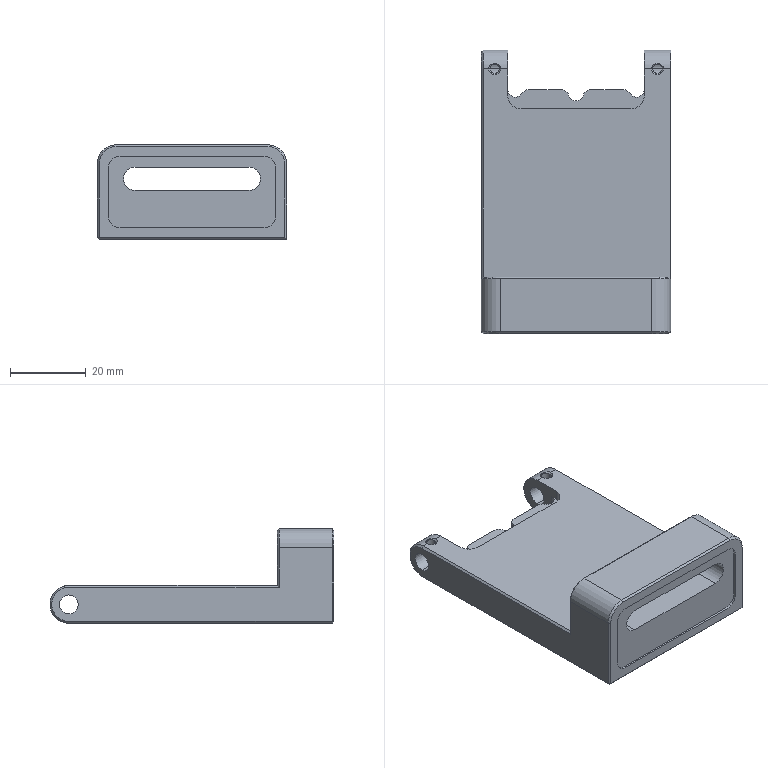Part | SolidWorks | features ICE 6, Chamfer 2, Fillet 2, Extrusion 1, HoleWzd 1, MoveFace 1 | 1 solid | 75 faces | box 50 x 75 x 25 mm | volume 33141 mm3 | plane 35 | cylinder 31 | cone 9 | commonest cylinder face diameters 4 x7 2.5 x4 5 x4 6 x4 7 x4 10 x4